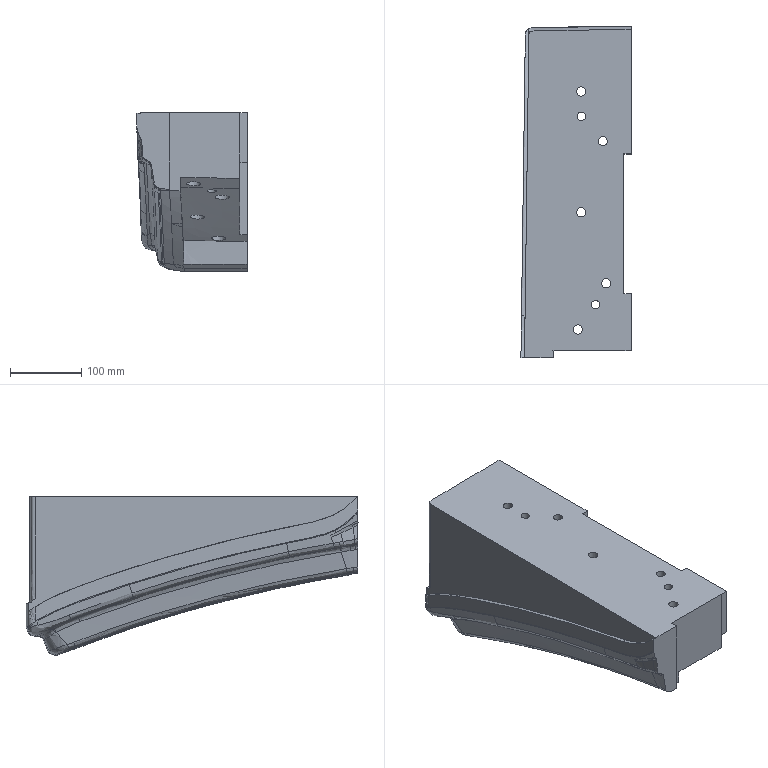Part | NX | features solid 2 | 1 solid | 126 faces | box 155.054 x 468.463 x 223.344 mm | volume 9677854 mm3 | spline 91 | plane 21 | cylinder 14 | commonest cylinder face diameters 13 x7 20 x5 12 x2